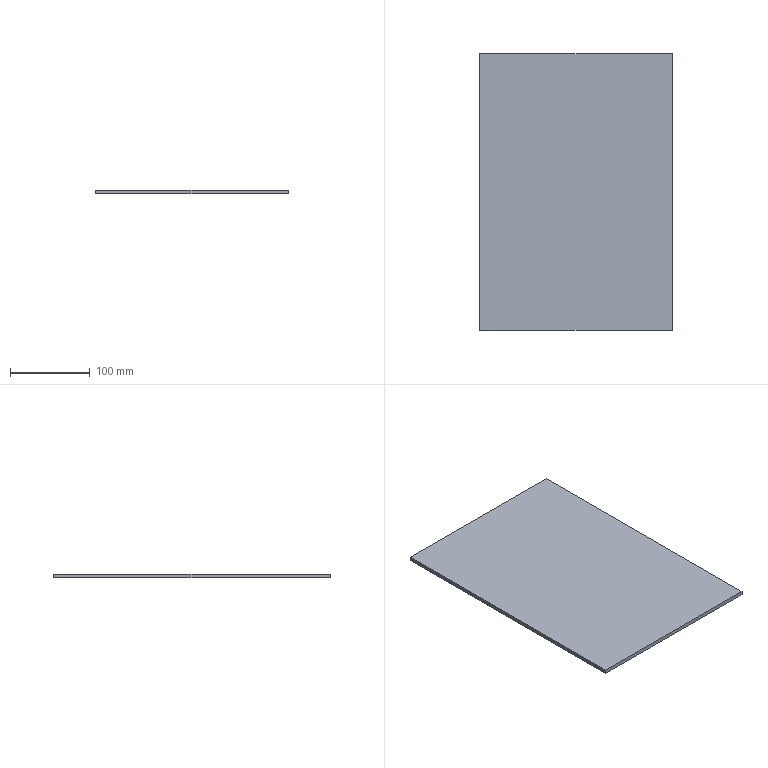Part | STEP file | MYT-A01-P26 | 1 solid | 6 faces | box 242 x 348 x 5 mm | volume 421080 mm3 | plane 6
STEP:
#1=CARTESIAN_POINT('',(121.,-174.,0.));
#2=VERTEX_POINT('',#1);
#3=CARTESIAN_POINT('',(121.,174.,0.));
#4=VERTEX_POINT('',#3);
#5=CARTESIAN_POINT('',(121.,174.,0.));
#6=DIRECTION('',(0.,1.,0.));
#7=VECTOR('',#6,1000.);
#8=LINE('',#5,#7);
#9=EDGE_CURVE('',#2,#4,#8,.T.);
#10=ORIENTED_EDGE('',*,*,#9,.T.);
#11=CARTESIAN_POINT('',(121.,174.,5.));
#12=VERTEX_POINT('',#11);
#13=CARTESIAN_POINT('',(121.,174.,5.));
#14=DIRECTION('',(0.,0.,-1.));
#15=VECTOR('',#14,1000.);
#16=LINE('',#13,#15);
#17=EDGE_CURVE('',#12,#4,#16,.T.);
#18=ORIENTED_EDGE('',*,*,#17,.F.);
#19=CARTESIAN_POINT('',(121.,-174.,5.));
#20=VERTEX_POINT('',#19);
#21=CARTESIAN_POINT('',(121.,174.,5.));
#22=DIRECTION('',(0.,1.,0.));
#23=VECTOR('',#22,1000.);
#24=LINE('',#21,#23);
#25=EDGE_CURVE('',#20,#12,#24,.T.);
#26=ORIENTED_EDGE('',*,*,#25,.F.);
#27=CARTESIAN_POINT('',(121.,-174.,5.));
#28=DIRECTION('',(0.,0.,-1.));
#29=VECTOR('',#28,1000.);
#30=LINE('',#27,#29);
#31=EDGE_CURVE('',#20,#2,#30,.T.);
#32=ORIENTED_EDGE('',*,*,#31,.T.);
#33=EDGE_LOOP('',(#10,#18,#26,#32));
#34=FACE_OUTER_BOUND('',#33,.T.);
#35=CARTESIAN_POINT('',(121.,174.,5.));
#36=DIRECTION('',(-1.,0.,0.));
#37=DIRECTION('',(0.,-1.,0.));
#38=AXIS2_PLACEMENT_3D('',#35,#36,#37);
#39=PLANE('',#38);
#40=ADVANCED_FACE('',(#34),#39,.F.);
#41=CARTESIAN_POINT('',(-121.,174.,0.));
#42=VERTEX_POINT('',#41);
#43=CARTESIAN_POINT('',(-121.,174.,0.));
#44=DIRECTION('',(-1.,0.,0.));
#45=VECTOR('',#44,1000.);
#46=LINE('',#43,#45);
#47=EDGE_CURVE('',#4,#42,#46,.T.);
#48=ORIENTED_EDGE('',*,*,#47,.T.);
#49=CARTESIAN_POINT('',(-121.,174.,5.));
#50=VERTEX_POINT('',#49);
#51=CARTESIAN_POINT('',(-121.,174.,5.));
#52=DIRECTION('',(0.,0.,-1.));
#53=VECTOR('',#52,1000.);
#54=LINE('',#51,#53);
#55=EDGE_CURVE('',#50,#42,#54,.T.);
#56=ORIENTED_EDGE('',*,*,#55,.F.);
#57=CARTESIAN_POINT('',(-121.,174.,5.));
#58=DIRECTION('',(-1.,0.,0.));
#59=VECTOR('',#58,1000.);
#60=LINE('',#57,#59);
#61=EDGE_CURVE('',#12,#50,#60,.T.);
#62=ORIENTED_EDGE('',*,*,#61,.F.);
#63=ORIENTED_EDGE('',*,*,#17,.T.);
#64=EDGE_LOOP('',(#48,#56,#62,#63));
#65=FACE_OUTER_BOUND('',#64,.T.);
#66=CARTESIAN_POINT('',(-121.,174.,5.));
#67=DIRECTION('',(0.,-1.,0.));
#68=DIRECTION('',(0.,0.,-1.));
#69=AXIS2_PLACEMENT_3D('',#66,#67,#68);
#70=PLANE('',#69);
#71=ADVANCED_FACE('',(#65),#70,.F.);
#72=CARTESIAN_POINT('',(-121.,-174.,0.));
#73=VERTEX_POINT('',#72);
#74=CARTESIAN_POINT('',(-121.,174.,0.));
#75=DIRECTION('',(0.,-1.,0.));
#76=VECTOR('',#75,1000.);
#77=LINE('',#74,#76);
#78=EDGE_CURVE('',#42,#73,#77,.T.);
#79=ORIENTED_EDGE('',*,*,#78,.T.);
#80=CARTESIAN_POINT('',(-121.,-174.,5.));
#81=VERTEX_POINT('',#80);
#82=CARTESIAN_POINT('',(-121.,-174.,5.));
#83=DIRECTION('',(0.,0.,-1.));
#84=VECTOR('',#83,1000.);
#85=LINE('',#82,#84);
#86=EDGE_CURVE('',#81,#73,#85,.T.);
#87=ORIENTED_EDGE('',*,*,#86,.F.);
#88=CARTESIAN_POINT('',(-121.,174.,5.));
#89=DIRECTION('',(0.,-1.,0.));
#90=VECTOR('',#89,1000.);
#91=LINE('',#88,#90);
#92=EDGE_CURVE('',#50,#81,#91,.T.);
#93=ORIENTED_EDGE('',*,*,#92,.F.);
#94=ORIENTED_EDGE('',*,*,#55,.T.);
#95=EDGE_LOOP('',(#79,#87,#93,#94));
#96=FACE_OUTER_BOUND('',#95,.T.);
#97=CARTESIAN_POINT('',(-121.,174.,5.));
#98=DIRECTION('',(1.,0.,0.));
#99=DIRECTION('',(0.,1.,0.));
#100=AXIS2_PLACEMENT_3D('',#97,#98,#99);
#101=PLANE('',#100);
#102=ADVANCED_FACE('',(#96),#101,.F.);
#103=CARTESIAN_POINT('',(-121.,-174.,0.));
#104=DIRECTION('',(1.,0.,0.));
#105=VECTOR('',#104,1000.);
#106=LINE('',#103,#105);
#107=EDGE_CURVE('',#73,#2,#106,.T.);
#108=ORIENTED_EDGE('',*,*,#107,.T.);
#109=ORIENTED_EDGE('',*,*,#31,.F.);
#110=CARTESIAN_POINT('',(-121.,-174.,5.));
#111=DIRECTION('',(1.,0.,0.));
#112=VECTOR('',#111,1000.);
#113=LINE('',#110,#112);
#114=EDGE_CURVE('',#81,#20,#113,.T.);
#115=ORIENTED_EDGE('',*,*,#114,.F.);
#116=ORIENTED_EDGE('',*,*,#86,.T.);
#117=EDGE_LOOP('',(#108,#109,#115,#116));
#118=FACE_OUTER_BOUND('',#117,.T.);
#119=CARTESIAN_POINT('',(-121.,-174.,5.));
#120=DIRECTION('',(0.,1.,0.));
#121=DIRECTION('',(0.,0.,1.));
#122=AXIS2_PLACEMENT_3D('',#119,#120,#121);
#123=PLANE('',#122);
#124=ADVANCED_FACE('',(#118),#123,.F.);
#125=ORIENTED_EDGE('',*,*,#25,.T.);
#126=ORIENTED_EDGE('',*,*,#61,.T.);
#127=ORIENTED_EDGE('',*,*,#92,.T.);
#128=ORIENTED_EDGE('',*,*,#114,.T.);
#129=EDGE_LOOP('',(#125,#126,#127,#128));
#130=FACE_OUTER_BOUND('',#129,.T.);
#131=CARTESIAN_POINT('',(0.,0.,5.));
#132=DIRECTION('',(0.,0.,1.));
#133=DIRECTION('',(1.,0.,0.));
#134=AXIS2_PLACEMENT_3D('',#131,#132,#133);
#135=PLANE('',#134);
#136=ADVANCED_FACE('',(#130),#135,.T.);
#137=ORIENTED_EDGE('',*,*,#9,.F.);
#138=ORIENTED_EDGE('',*,*,#107,.F.);
#139=ORIENTED_EDGE('',*,*,#78,.F.);
#140=ORIENTED_EDGE('',*,*,#47,.F.);
#141=EDGE_LOOP('',(#137,#138,#139,#140));
#142=FACE_OUTER_BOUND('',#141,.T.);
#143=CARTESIAN_POINT('',(0.,0.,0.));
#144=DIRECTION('',(0.,0.,1.));
#145=DIRECTION('',(1.,0.,0.));
#146=AXIS2_PLACEMENT_3D('',#143,#144,#145);
#147=PLANE('',#146);
#148=ADVANCED_FACE('',(#142),#147,.F.);
#149=CLOSED_SHELL('',(#40,#71,#102,#124,#136,#148));
#150=MANIFOLD_SOLID_BREP('',#149);
#151=CARTESIAN_POINT('',(0.,0.,0.));
#152=DIRECTION('',(0.,0.,1.));
#153=DIRECTION('',(1.,0.,0.));
#154=AXIS2_PLACEMENT_3D('',#151,#152,#153);
#155=(LENGTH_UNIT()NAMED_UNIT(*)SI_UNIT(.MILLI.,.METRE.));
#156=UNCERTAINTY_MEASURE_WITH_UNIT(LENGTH_MEASURE(0.00001),#155,'','');
#157=(NAMED_UNIT(*)PLANE_ANGLE_UNIT()SI_UNIT($,.RADIAN.));
#158=(NAMED_UNIT(*)SI_UNIT($,.STERADIAN.)SOLID_ANGLE_UNIT());
#159=(GEOMETRIC_REPRESENTATION_CONTEXT(3)GLOBAL_UNCERTAINTY_ASSIGNED_CONTEXT((#156))GLOBAL_UNIT_ASSIGNED_CONTEXT((#155,#157,#158))REPRESENTATION_CONTEXT('',''));
#160=ADVANCED_BREP_SHAPE_REPRESENTATION('',(#150,#154),#159);